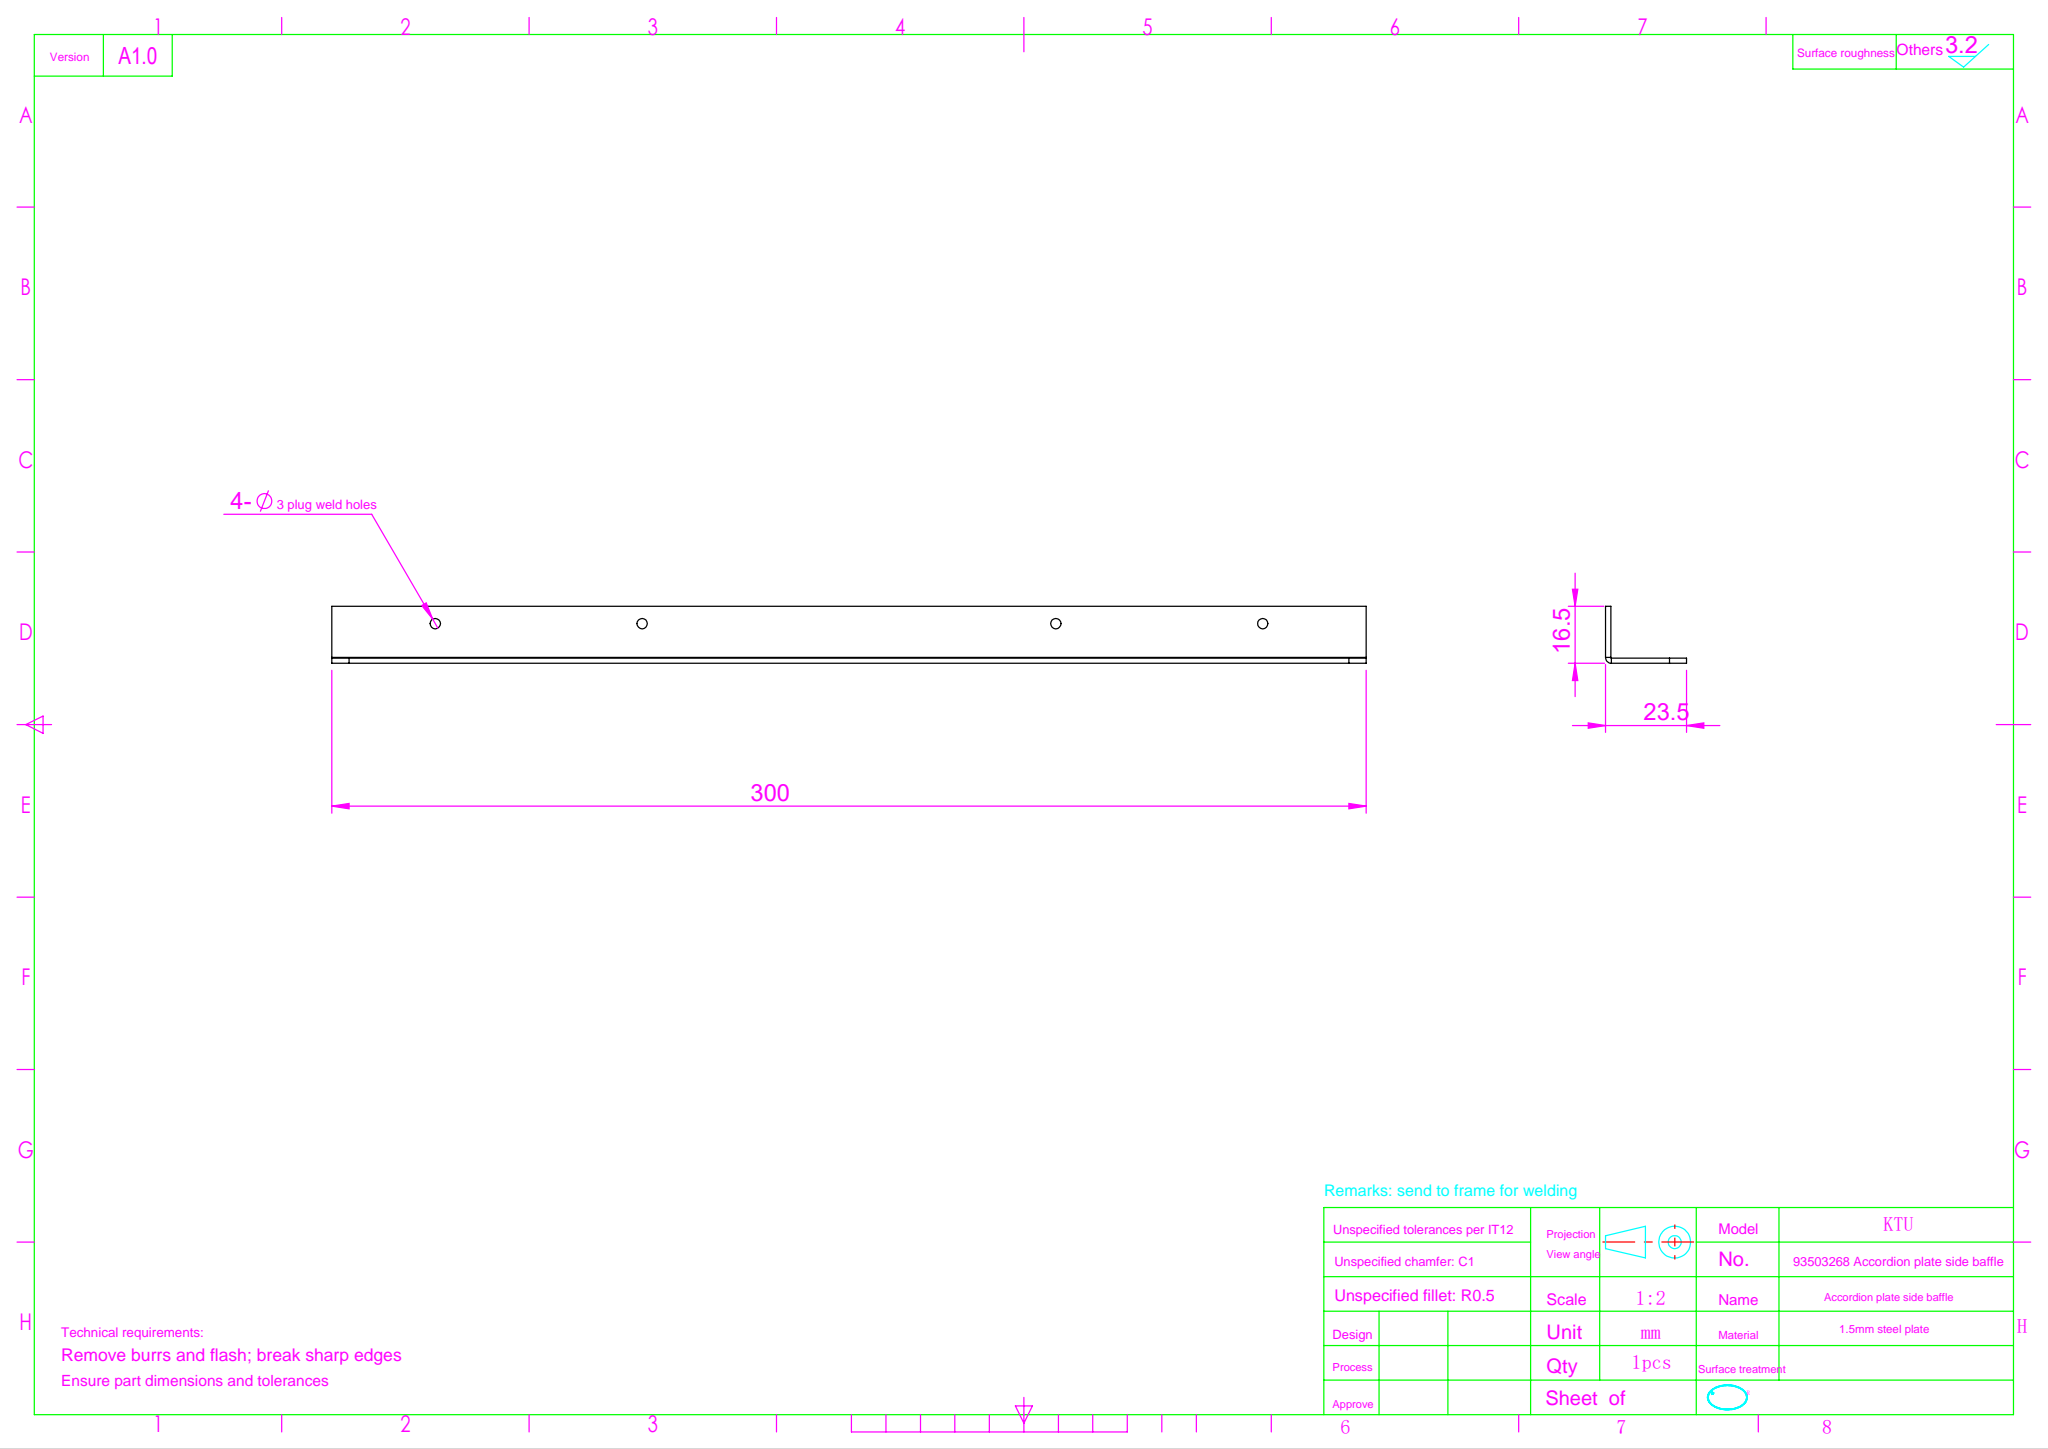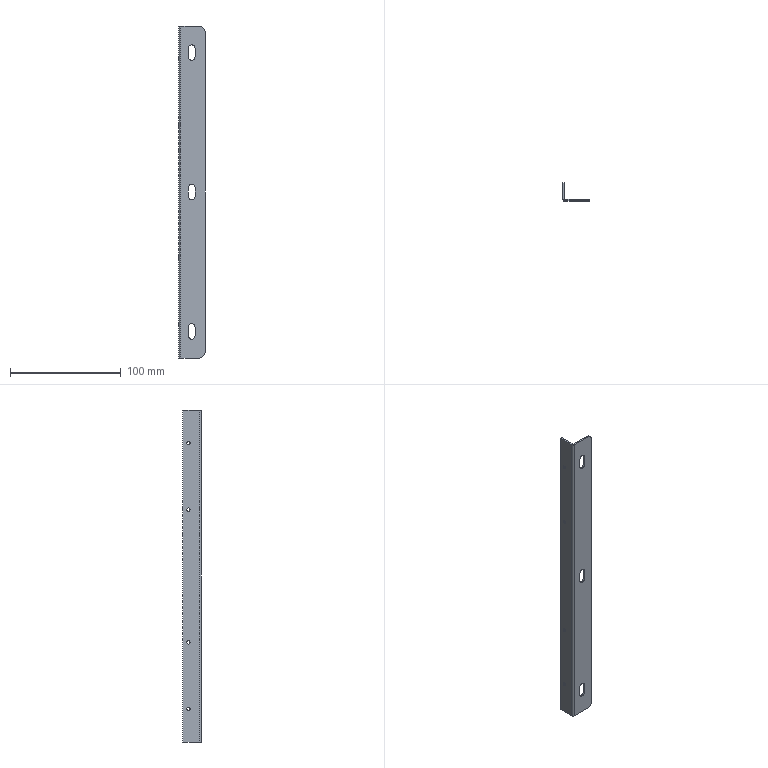Part | SolidWorks | features ICE 2, Fillet 1, FlatPattern 1, SMBaseFlange 1, SheetMetal 1 | 1 solid | 39 faces | box 23.5 x 16.5 x 300 mm | volume 16740 mm3 | cylinder 21 | plane 18 | commonest cylinder face diameters 6 x9 3 x8 10 x2 0.4 x1 3.4 x1